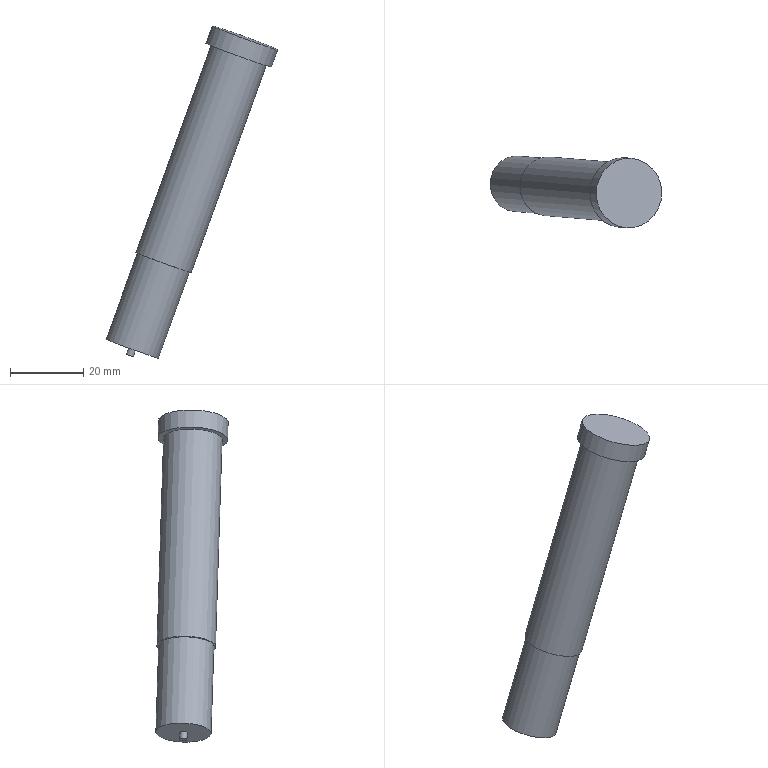Part | NX | features solid 2 | 1 solid | 9 faces | box 46.694 x 19.725 x 90.404 mm | volume 17965 mm3 | plane 5 | cylinder 4 | commonest cylinder face diameters 2 x1 15.1 x1 16 x1 19 x1
STEP:
#1=CARTESIAN_POINT('',(495.973,91.683,-28.285));
#2=VERTEX_POINT('',#1);
#3=CARTESIAN_POINT('',(495.276,83.714,-28.285));
#4=DIRECTION('',(0.3407,-0.02981,0.9397));
#5=DIRECTION('',(0.08716,0.9962,0.));
#6=AXIS2_PLACEMENT_3D('',#3,#4,#5);
#7=CIRCLE('',#6,8.);
#8=EDGE_CURVE('',#2,#2,#7,.T.);
#9=ORIENTED_EDGE('',*,*,#8,.T.);
#10=EDGE_LOOP('',(#9));
#11=FACE_BOUND('',#10,.T.);
#12=CARTESIAN_POINT('',(516.416,89.895,28.096));
#13=VERTEX_POINT('',#12);
#14=CARTESIAN_POINT('',(515.719,81.925,28.096));
#15=DIRECTION('',(0.3407,-0.02981,0.9397));
#16=DIRECTION('',(0.08716,0.9962,0.));
#17=AXIS2_PLACEMENT_3D('',#14,#15,#16);
#18=CIRCLE('',#17,8.);
#19=EDGE_CURVE('',#13,#13,#18,.T.);
#20=ORIENTED_EDGE('',*,*,#19,.F.);
#21=EDGE_LOOP('',(#20));
#22=FACE_BOUND('',#21,.T.);
#23=CARTESIAN_POINT('',(517.423,81.776,32.795));
#24=DIRECTION('',(-0.3407,0.02981,-0.9397));
#25=DIRECTION('',(-0.08716,-0.9962,0.));
#26=AXIS2_PLACEMENT_3D('',#23,#24,#25);
#27=CYLINDRICAL_SURFACE('',#26,8.);
#28=ADVANCED_FACE('',(#11,#22),#27,.T.);
#29=CARTESIAN_POINT('',(495.934,91.235,-28.285));
#30=VERTEX_POINT('',#29);
#31=CARTESIAN_POINT('',(495.276,83.714,-28.285));
#32=DIRECTION('',(0.3407,-0.02981,0.9397));
#33=DIRECTION('',(0.08716,0.9962,0.));
#34=AXIS2_PLACEMENT_3D('',#31,#32,#33);
#35=CIRCLE('',#34,7.55);
#36=EDGE_CURVE('',#30,#30,#35,.T.);
#37=ORIENTED_EDGE('',*,*,#36,.T.);
#38=EDGE_LOOP('',(#37));
#39=FACE_BOUND('',#38,.T.);
#40=ORIENTED_EDGE('',*,*,#8,.F.);
#41=EDGE_LOOP('',(#40));
#42=FACE_BOUND('',#41,.T.);
#43=CARTESIAN_POINT('',(495.276,83.714,-28.285));
#44=DIRECTION('',(0.3407,-0.02981,0.9397));
#45=DIRECTION('',(0.08716,0.9962,0.));
#46=AXIS2_PLACEMENT_3D('',#43,#44,#45);
#47=PLANE('',#46);
#48=ADVANCED_FACE('',(#39,#42),#47,.F.);
#49=CARTESIAN_POINT('',(516.547,91.389,28.096));
#50=VERTEX_POINT('',#49);
#51=CARTESIAN_POINT('',(515.719,81.925,28.096));
#52=DIRECTION('',(0.3407,-0.02981,0.9397));
#53=DIRECTION('',(0.08716,0.9962,0.));
#54=AXIS2_PLACEMENT_3D('',#51,#52,#53);
#55=CIRCLE('',#54,9.5);
#56=EDGE_CURVE('',#50,#50,#55,.T.);
#57=ORIENTED_EDGE('',*,*,#56,.F.);
#58=EDGE_LOOP('',(#57));
#59=FACE_BOUND('',#58,.T.);
#60=ORIENTED_EDGE('',*,*,#19,.T.);
#61=EDGE_LOOP('',(#60));
#62=FACE_BOUND('',#61,.T.);
#63=CARTESIAN_POINT('',(515.719,81.925,28.096));
#64=DIRECTION('',(0.3407,-0.02981,0.9397));
#65=DIRECTION('',(0.08716,0.9962,0.));
#66=AXIS2_PLACEMENT_3D('',#63,#64,#65);
#67=PLANE('',#66);
#68=ADVANCED_FACE('',(#59,#62),#67,.F.);
#69=ORIENTED_EDGE('',*,*,#56,.T.);
#70=EDGE_LOOP('',(#69));
#71=FACE_BOUND('',#70,.T.);
#72=CARTESIAN_POINT('',(518.251,91.24,32.795));
#73=VERTEX_POINT('',#72);
#74=CARTESIAN_POINT('',(517.423,81.776,32.795));
#75=DIRECTION('',(0.3407,-0.02981,0.9397));
#76=DIRECTION('',(0.08716,0.9962,0.));
#77=AXIS2_PLACEMENT_3D('',#74,#75,#76);
#78=CIRCLE('',#77,9.5);
#79=EDGE_CURVE('',#73,#73,#78,.T.);
#80=ORIENTED_EDGE('',*,*,#79,.F.);
#81=EDGE_LOOP('',(#80));
#82=FACE_BOUND('',#81,.T.);
#83=CARTESIAN_POINT('',(515.719,81.925,28.096));
#84=DIRECTION('',(0.3407,-0.02981,0.9397));
#85=DIRECTION('',(0.08716,0.9962,0.));
#86=AXIS2_PLACEMENT_3D('',#83,#84,#85);
#87=CYLINDRICAL_SURFACE('',#86,9.5);
#88=ADVANCED_FACE('',(#71,#82),#87,.T.);
#89=ORIENTED_EDGE('',*,*,#79,.T.);
#90=EDGE_LOOP('',(#89));
#91=FACE_BOUND('',#90,.T.);
#92=CARTESIAN_POINT('',(517.423,81.776,32.795));
#93=DIRECTION('',(0.3407,-0.02981,0.9397));
#94=DIRECTION('',(0.08716,0.9962,0.));
#95=AXIS2_PLACEMENT_3D('',#92,#93,#94);
#96=PLANE('',#95);
#97=ADVANCED_FACE('',(#91),#96,.T.);
#98=CARTESIAN_POINT('',(487.416,91.98,-51.778));
#99=VERTEX_POINT('',#98);
#100=CARTESIAN_POINT('',(486.758,84.459,-51.778));
#101=DIRECTION('',(0.3407,-0.02981,0.9397));
#102=DIRECTION('',(0.08716,0.9962,0.));
#103=AXIS2_PLACEMENT_3D('',#100,#101,#102);
#104=CIRCLE('',#103,7.55);
#105=EDGE_CURVE('',#99,#99,#104,.T.);
#106=ORIENTED_EDGE('',*,*,#105,.T.);
#107=EDGE_LOOP('',(#106));
#108=FACE_BOUND('',#107,.T.);
#109=ORIENTED_EDGE('',*,*,#36,.F.);
#110=EDGE_LOOP('',(#109));
#111=FACE_BOUND('',#110,.T.);
#112=CARTESIAN_POINT('',(486.758,84.459,-51.778));
#113=DIRECTION('',(0.3407,-0.02981,0.9397));
#114=DIRECTION('',(0.08716,0.9962,0.));
#115=AXIS2_PLACEMENT_3D('',#112,#113,#114);
#116=CYLINDRICAL_SURFACE('',#115,7.55);
#117=ADVANCED_FACE('',(#108,#111),#116,.T.);
#118=CARTESIAN_POINT('',(486.845,85.455,-51.778));
#119=VERTEX_POINT('',#118);
#120=CARTESIAN_POINT('',(486.758,84.459,-51.778));
#121=DIRECTION('',(0.3407,-0.02981,0.9397));
#122=DIRECTION('',(0.08716,0.9962,0.));
#123=AXIS2_PLACEMENT_3D('',#120,#121,#122);
#124=CIRCLE('',#123,1.);
#125=EDGE_CURVE('',#119,#119,#124,.T.);
#126=ORIENTED_EDGE('',*,*,#125,.T.);
#127=EDGE_LOOP('',(#126));
#128=FACE_BOUND('',#127,.T.);
#129=ORIENTED_EDGE('',*,*,#105,.F.);
#130=EDGE_LOOP('',(#129));
#131=FACE_BOUND('',#130,.T.);
#132=CARTESIAN_POINT('',(486.758,84.459,-51.778));
#133=DIRECTION('',(0.3407,-0.02981,0.9397));
#134=DIRECTION('',(0.08716,0.9962,0.));
#135=AXIS2_PLACEMENT_3D('',#132,#133,#134);
#136=PLANE('',#135);
#137=ADVANCED_FACE('',(#128,#131),#136,.F.);
#138=CARTESIAN_POINT('',(486.164,85.515,-53.657));
#139=VERTEX_POINT('',#138);
#140=CARTESIAN_POINT('',(486.077,84.519,-53.657));
#141=DIRECTION('',(0.3407,-0.02981,0.9397));
#142=DIRECTION('',(0.08716,0.9962,0.));
#143=AXIS2_PLACEMENT_3D('',#140,#141,#142);
#144=CIRCLE('',#143,1.);
#145=EDGE_CURVE('',#139,#139,#144,.T.);
#146=ORIENTED_EDGE('',*,*,#145,.T.);
#147=EDGE_LOOP('',(#146));
#148=FACE_BOUND('',#147,.T.);
#149=ORIENTED_EDGE('',*,*,#125,.F.);
#150=EDGE_LOOP('',(#149));
#151=FACE_BOUND('',#150,.T.);
#152=CARTESIAN_POINT('',(486.077,84.519,-53.657));
#153=DIRECTION('',(0.3407,-0.02981,0.9397));
#154=DIRECTION('',(0.08716,0.9962,0.));
#155=AXIS2_PLACEMENT_3D('',#152,#153,#154);
#156=CYLINDRICAL_SURFACE('',#155,1.);
#157=ADVANCED_FACE('',(#148,#151),#156,.T.);
#158=ORIENTED_EDGE('',*,*,#145,.F.);
#159=EDGE_LOOP('',(#158));
#160=FACE_BOUND('',#159,.T.);
#161=CARTESIAN_POINT('',(486.077,84.519,-53.657));
#162=DIRECTION('',(0.3407,-0.02981,0.9397));
#163=DIRECTION('',(0.08716,0.9962,0.));
#164=AXIS2_PLACEMENT_3D('',#161,#162,#163);
#165=PLANE('',#164);
#166=ADVANCED_FACE('',(#160),#165,.F.);
#167=CLOSED_SHELL('',(#28,#48,#68,#88,#97,#117,#137,#157,#166));
#168=MANIFOLD_SOLID_BREP('',#167);
#169=(LENGTH_UNIT()NAMED_UNIT(*)SI_UNIT(.MILLI.,.METRE.));
#170=UNCERTAINTY_MEASURE_WITH_UNIT(LENGTH_MEASURE(0.00001),#169,'','');
#171=(NAMED_UNIT(*)PLANE_ANGLE_UNIT()SI_UNIT($,.RADIAN.));
#172=(NAMED_UNIT(*)SI_UNIT($,.STERADIAN.)SOLID_ANGLE_UNIT());
#173=(GEOMETRIC_REPRESENTATION_CONTEXT(3)GLOBAL_UNCERTAINTY_ASSIGNED_CONTEXT((#170))GLOBAL_UNIT_ASSIGNED_CONTEXT((#169,#171,#172))REPRESENTATION_CONTEXT('',''));
#174=ADVANCED_BREP_SHAPE_REPRESENTATION('',(#168),#173);